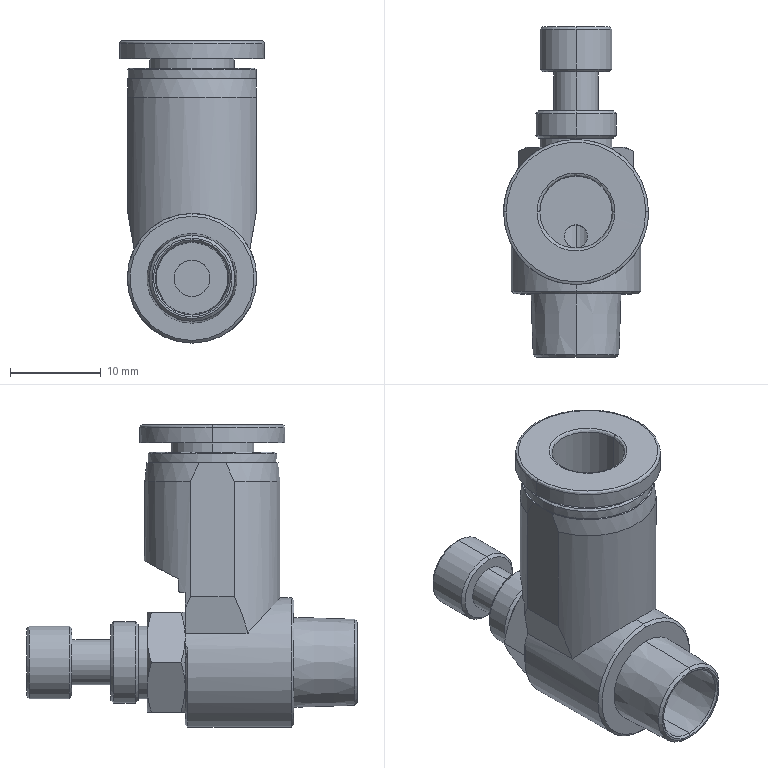Part | STEP file | KZB668-08-01-668 | 1 solid | 105 faces | box 16 x 36.5 x 33.35 mm | volume 5183 mm3 | cone 42 | plane 32 | cylinder 27 | spline 4 | commonest cylinder face diameters 8 x6 15 x4 2.567 x2 4 x2 5 x2 9 x2